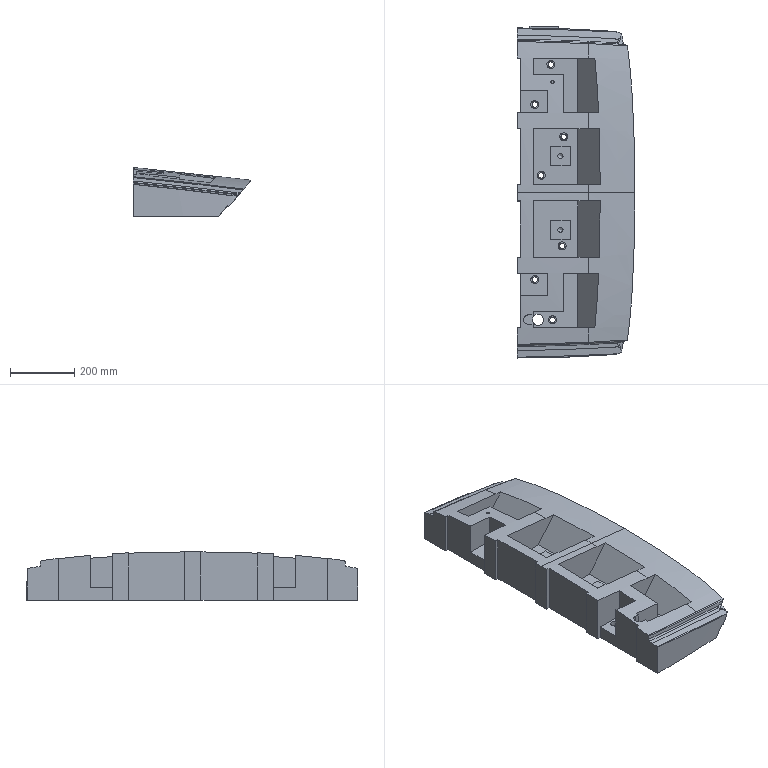Part | NX | features solid 2 | 1 solid | 166 faces | box 366.676 x 1034 x 152.113 mm | volume 28384770 mm3 | plane 77 | spline 60 | cylinder 27 | cone 2 | commonest cylinder face diameters 20 x8 17 x7 25 x7 16 x2 10 x1 30 x1